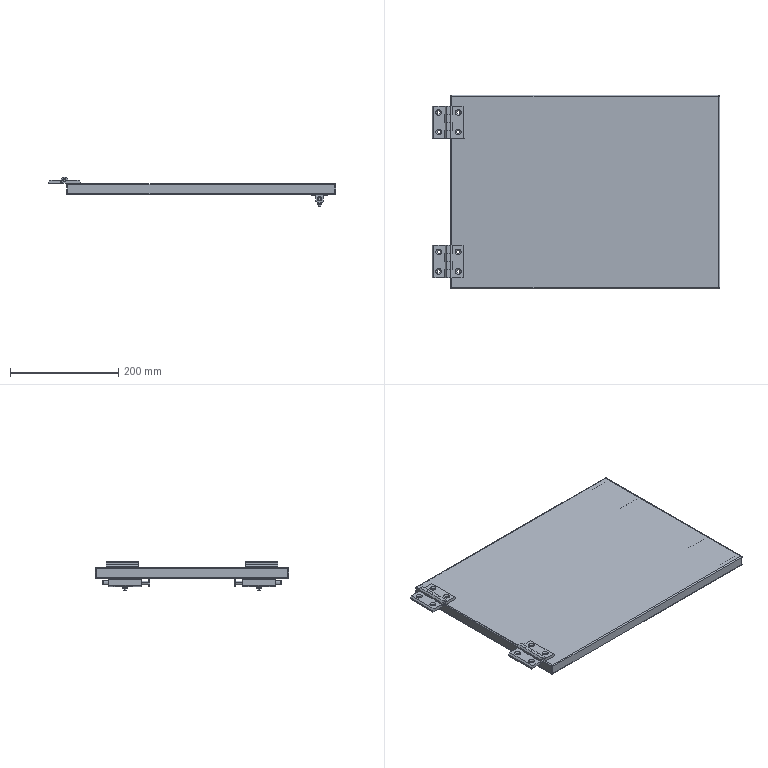Part | SolidWorks | 17 solids | 416 faces | box 532 x 358 x 55 mm | volume 405860 mm3 | plane 196 | cylinder 144 | cone 40 | spline 20 | sphere 16 | commonest cylinder face diameters 2 x20 4 x20 5.8 x20 3.4 x16 6.4 x16 8 x12